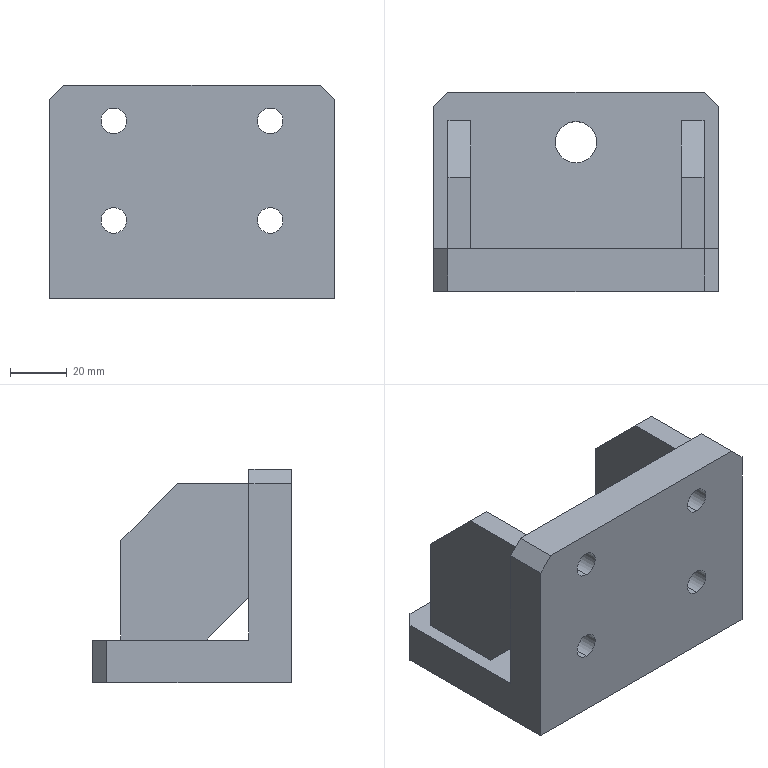Part | STEP file | YCD14007A-08.02.05-Lift Cylinder Connecting Plate-A3_Default<Machined> | 1 solid | 34 faces | box 100 x 70 x 75 mm | volume 222556 mm3 | plane 24 | cylinder 10 | commonest cylinder face diameters 9 x8 14.5 x2